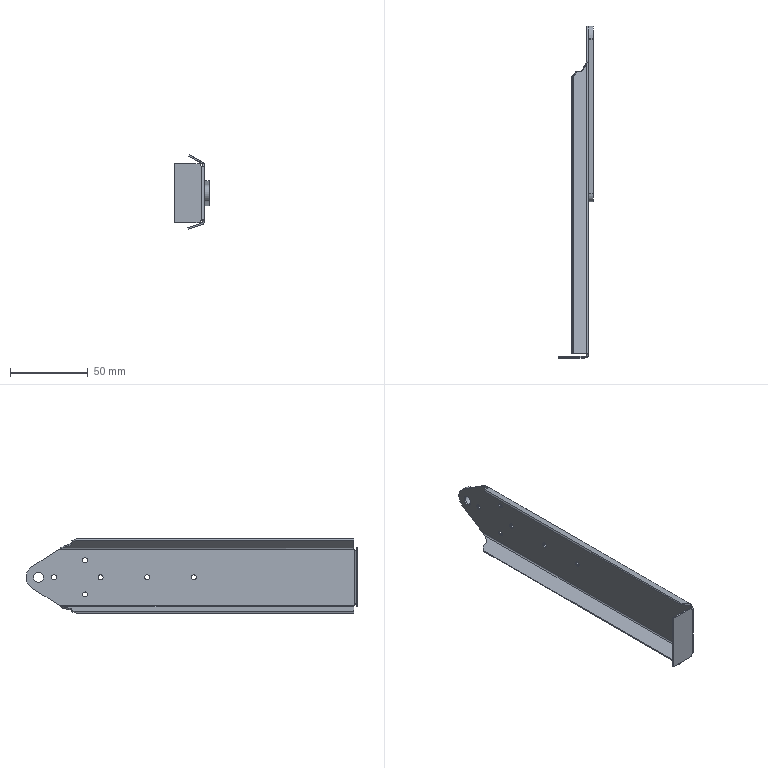Part | SolidWorks | features BaseBody 2 | 2 solids | 74 faces | box 22.422 x 213.802 x 48.105 mm | volume 16813 mm3 | cylinder 41 | plane 27 | spline 6 | commonest cylinder face diameters 3.2 x20 4 x7 6.35 x4 16 x4 2 x3 5 x2